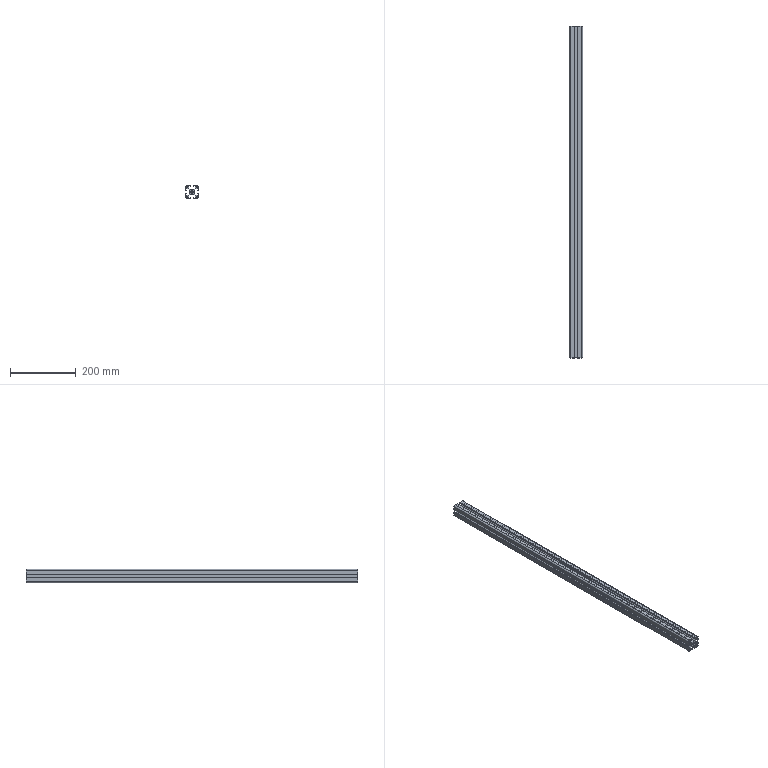Part | SolidWorks | features WeldMemberFeat 1, WeldmentFeature 1 | 1 solid | 92 faces | box 40 x 1013 x 40 mm | volume 612706 mm3 | plane 78 | cylinder 14 | commonest cylinder face diameters 6 x8 9 x4 6.8 x2